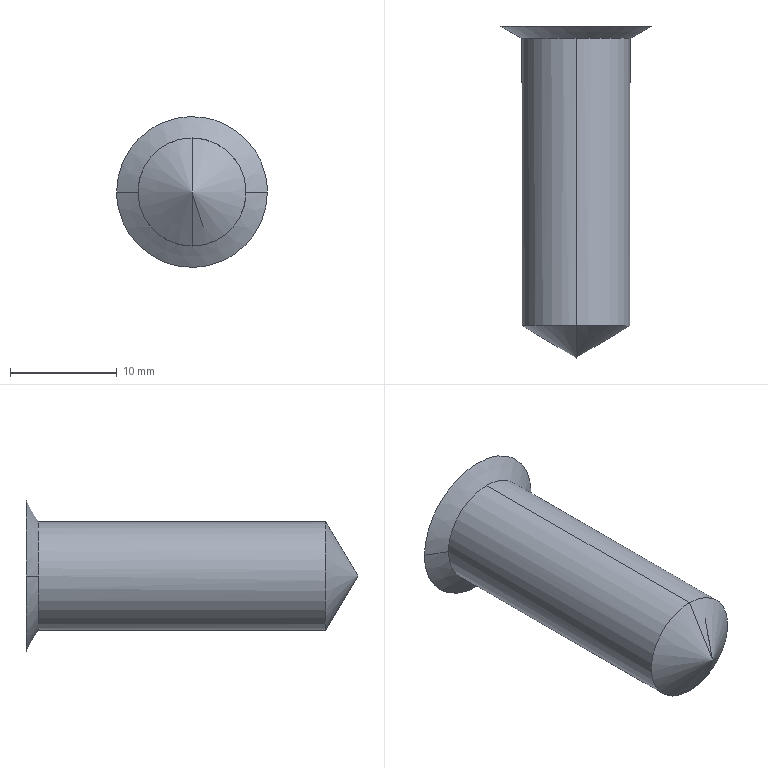Part | NX | features solid 2 | 1 solid | 7 faces | box 14.106 x 31.036 x 14.106 mm | volume 2368 mm3 | cone 4 | cylinder 2 | plane 1 | commonest cylinder face diameters 10.106 x2
STEP:
#1=CARTESIAN_POINT('',(-165.,-29.,-162.053));
#2=VERTEX_POINT('',#1);
#3=CARTESIAN_POINT('',(-165.,-2.155,-162.053));
#4=VERTEX_POINT('',#3);
#5=CARTESIAN_POINT('',(-165.,-29.,-162.053));
#6=CARTESIAN_POINT('',(-165.,-20.052,-162.053));
#7=CARTESIAN_POINT('',(-165.,-11.103,-162.053));
#8=CARTESIAN_POINT('',(-165.,-2.155,-162.053));
#9=B_SPLINE_CURVE_WITH_KNOTS('',3,(#5,#6,#7,#8),.UNSPECIFIED.,.F.,.F.,(4,4),(0.,1.),.UNSPECIFIED.);
#10=EDGE_CURVE('',#2,#4,#9,.T.);
#11=ORIENTED_EDGE('',*,*,#10,.T.);
#12=CARTESIAN_POINT('',(-159.947,-2.155,-157.));
#13=VERTEX_POINT('',#12);
#14=CARTESIAN_POINT('',(-165.,-2.155,-162.053));
#15=CARTESIAN_POINT('',(-163.677,-2.155,-162.053));
#16=CARTESIAN_POINT('',(-161.042,-2.155,-160.958));
#17=CARTESIAN_POINT('',(-159.947,-2.155,-158.323));
#18=CARTESIAN_POINT('',(-159.947,-2.155,-157.));
#19=B_SPLINE_CURVE_WITH_KNOTS('',3,(#14,#15,#16,#17,#18),.UNSPECIFIED.,.F.,.F.,(4,1,4),(0.,0.5,1.),.UNSPECIFIED.);
#20=EDGE_CURVE('',#4,#13,#19,.T.);
#21=ORIENTED_EDGE('',*,*,#20,.T.);
#22=CARTESIAN_POINT('',(-165.,-2.155,-151.947));
#23=VERTEX_POINT('',#22);
#24=CARTESIAN_POINT('',(-159.947,-2.155,-157.));
#25=CARTESIAN_POINT('',(-159.947,-2.155,-155.677));
#26=CARTESIAN_POINT('',(-161.042,-2.155,-153.042));
#27=CARTESIAN_POINT('',(-163.677,-2.155,-151.947));
#28=CARTESIAN_POINT('',(-165.,-2.155,-151.947));
#29=B_SPLINE_CURVE_WITH_KNOTS('',3,(#24,#25,#26,#27,#28),.UNSPECIFIED.,.F.,.F.,(4,1,4),(0.,0.5,1.),.UNSPECIFIED.);
#30=EDGE_CURVE('',#13,#23,#29,.T.);
#31=ORIENTED_EDGE('',*,*,#30,.T.);
#32=CARTESIAN_POINT('',(-165.,-29.,-151.947));
#33=VERTEX_POINT('',#32);
#34=CARTESIAN_POINT('',(-165.,-2.155,-151.947));
#35=CARTESIAN_POINT('',(-165.,-11.103,-151.947));
#36=CARTESIAN_POINT('',(-165.,-20.052,-151.947));
#37=CARTESIAN_POINT('',(-165.,-29.,-151.947));
#38=B_SPLINE_CURVE_WITH_KNOTS('',3,(#34,#35,#36,#37),.UNSPECIFIED.,.F.,.F.,(4,4),(0.,1.),.UNSPECIFIED.);
#39=EDGE_CURVE('',#23,#33,#38,.T.);
#40=ORIENTED_EDGE('',*,*,#39,.T.);
#41=CARTESIAN_POINT('',(-165.,-29.,-151.947));
#42=CARTESIAN_POINT('',(-163.677,-29.,-151.947));
#43=CARTESIAN_POINT('',(-161.042,-29.,-153.04));
#44=CARTESIAN_POINT('',(-159.4,-29.,-157.));
#45=CARTESIAN_POINT('',(-161.042,-29.,-160.96));
#46=CARTESIAN_POINT('',(-163.677,-29.,-162.053));
#47=CARTESIAN_POINT('',(-165.,-29.,-162.053));
#48=B_SPLINE_CURVE_WITH_KNOTS('',3,(#41,#42,#43,#44,#45,#46,#47),.UNSPECIFIED.,.F.,.F.,(4,1,1,1,4),(0.,0.25,0.5,0.75,1.),.UNSPECIFIED.);
#49=EDGE_CURVE('',#33,#2,#48,.T.);
#50=ORIENTED_EDGE('',*,*,#49,.T.);
#51=EDGE_LOOP('',(#11,#21,#31,#40,#50));
#52=FACE_BOUND('',#51,.T.);
#53=CARTESIAN_POINT('',(-165.,-1.,-157.));
#54=DIRECTION('',(0.,-1.,0.));
#55=DIRECTION('',(0.,0.,1.));
#56=AXIS2_PLACEMENT_3D('',#53,#54,#55);
#57=CYLINDRICAL_SURFACE('',#56,5.053);
#58=ADVANCED_FACE('',(#52),#57,.T.);
#59=CARTESIAN_POINT('',(-157.947,-1.,-157.));
#60=VERTEX_POINT('',#59);
#61=CARTESIAN_POINT('',(-157.947,-1.,-157.));
#62=CARTESIAN_POINT('',(-158.614,-1.385,-157.));
#63=CARTESIAN_POINT('',(-159.28,-1.77,-157.));
#64=CARTESIAN_POINT('',(-159.947,-2.155,-157.));
#65=B_SPLINE_CURVE_WITH_KNOTS('',3,(#61,#62,#63,#64),.UNSPECIFIED.,.F.,.F.,(4,4),(0.,1.),.UNSPECIFIED.);
#66=EDGE_CURVE('',#60,#13,#65,.T.);
#67=ORIENTED_EDGE('',*,*,#66,.T.);
#68=ORIENTED_EDGE('',*,*,#20,.F.);
#69=CARTESIAN_POINT('',(-170.053,-2.155,-157.));
#70=VERTEX_POINT('',#69);
#71=CARTESIAN_POINT('',(-170.053,-2.155,-157.));
#72=CARTESIAN_POINT('',(-170.053,-2.155,-158.323));
#73=CARTESIAN_POINT('',(-168.958,-2.155,-160.958));
#74=CARTESIAN_POINT('',(-166.323,-2.155,-162.053));
#75=CARTESIAN_POINT('',(-165.,-2.155,-162.053));
#76=B_SPLINE_CURVE_WITH_KNOTS('',3,(#71,#72,#73,#74,#75),.UNSPECIFIED.,.F.,.F.,(4,1,4),(0.,0.5,1.),.UNSPECIFIED.);
#77=EDGE_CURVE('',#4,#70,#76,.F.);
#78=ORIENTED_EDGE('',*,*,#77,.T.);
#79=CARTESIAN_POINT('',(-172.053,-1.,-157.));
#80=VERTEX_POINT('',#79);
#81=CARTESIAN_POINT('',(-170.053,-2.155,-157.));
#82=CARTESIAN_POINT('',(-170.72,-1.77,-157.));
#83=CARTESIAN_POINT('',(-171.386,-1.385,-157.));
#84=CARTESIAN_POINT('',(-172.053,-1.,-157.));
#85=B_SPLINE_CURVE_WITH_KNOTS('',3,(#81,#82,#83,#84),.UNSPECIFIED.,.F.,.F.,(4,4),(0.,1.),.UNSPECIFIED.);
#86=EDGE_CURVE('',#70,#80,#85,.T.);
#87=ORIENTED_EDGE('',*,*,#86,.T.);
#88=CARTESIAN_POINT('',(-157.947,-1.,-157.));
#89=CARTESIAN_POINT('',(-157.947,-1.,-158.852));
#90=CARTESIAN_POINT('',(-159.473,-1.,-162.522));
#91=CARTESIAN_POINT('',(-165.,-1.,-164.819));
#92=CARTESIAN_POINT('',(-170.527,-1.,-162.521));
#93=CARTESIAN_POINT('',(-172.053,-1.,-158.853));
#94=CARTESIAN_POINT('',(-172.053,-1.,-157.));
#95=B_SPLINE_CURVE_WITH_KNOTS('',3,(#88,#89,#90,#91,#92,#93,#94),.UNSPECIFIED.,.F.,.F.,(4,1,1,1,4),(0.,0.25,0.5,0.75,1.),.UNSPECIFIED.);
#96=EDGE_CURVE('',#80,#60,#95,.F.);
#97=ORIENTED_EDGE('',*,*,#96,.T.);
#98=EDGE_LOOP('',(#67,#68,#78,#87,#97));
#99=FACE_BOUND('',#98,.T.);
#100=CARTESIAN_POINT('',(-165.,-1.,-157.));
#101=DIRECTION('',(0.,1.,0.));
#102=DIRECTION('',(-1.,0.,0.));
#103=AXIS2_PLACEMENT_3D('',#100,#101,#102);
#104=CONICAL_SURFACE('',#103,7.053,1.047);
#105=ADVANCED_FACE('',(#99),#104,.T.);
#106=ORIENTED_EDGE('',*,*,#77,.F.);
#107=ORIENTED_EDGE('',*,*,#10,.F.);
#108=CARTESIAN_POINT('',(-165.,-29.,-162.053));
#109=CARTESIAN_POINT('',(-166.323,-29.,-162.053));
#110=CARTESIAN_POINT('',(-168.958,-29.,-160.96));
#111=CARTESIAN_POINT('',(-170.6,-29.,-157.));
#112=CARTESIAN_POINT('',(-168.958,-29.,-153.04));
#113=CARTESIAN_POINT('',(-166.323,-29.,-151.947));
#114=CARTESIAN_POINT('',(-165.,-29.,-151.947));
#115=B_SPLINE_CURVE_WITH_KNOTS('',3,(#108,#109,#110,#111,#112,#113,#114),.UNSPECIFIED.,.F.,.F.,(4,1,1,1,4),(0.,0.25,0.5,0.75,1.),.UNSPECIFIED.);
#116=EDGE_CURVE('',#2,#33,#115,.T.);
#117=ORIENTED_EDGE('',*,*,#116,.T.);
#118=ORIENTED_EDGE('',*,*,#39,.F.);
#119=CARTESIAN_POINT('',(-165.,-2.155,-151.947));
#120=CARTESIAN_POINT('',(-166.323,-2.155,-151.947));
#121=CARTESIAN_POINT('',(-168.958,-2.155,-153.042));
#122=CARTESIAN_POINT('',(-170.053,-2.155,-155.677));
#123=CARTESIAN_POINT('',(-170.053,-2.155,-157.));
#124=B_SPLINE_CURVE_WITH_KNOTS('',3,(#119,#120,#121,#122,#123),.UNSPECIFIED.,.F.,.F.,(4,1,4),(0.,0.5,1.),.UNSPECIFIED.);
#125=EDGE_CURVE('',#23,#70,#124,.T.);
#126=ORIENTED_EDGE('',*,*,#125,.T.);
#127=EDGE_LOOP('',(#106,#107,#117,#118,#126));
#128=FACE_BOUND('',#127,.T.);
#129=CARTESIAN_POINT('',(-165.,-1.,-157.));
#130=DIRECTION('',(0.,-1.,0.));
#131=DIRECTION('',(0.,0.,1.));
#132=AXIS2_PLACEMENT_3D('',#129,#130,#131);
#133=CYLINDRICAL_SURFACE('',#132,5.053);
#134=ADVANCED_FACE('',(#128),#133,.T.);
#135=CARTESIAN_POINT('',(-165.,-32.036,-157.));
#136=VERTEX_POINT('',#135);
#137=CARTESIAN_POINT('',(-165.,-29.,-151.947));
#138=CARTESIAN_POINT('',(-165.,-30.012,-153.631));
#139=CARTESIAN_POINT('',(-165.,-31.024,-155.316));
#140=CARTESIAN_POINT('',(-165.,-32.036,-157.));
#141=B_SPLINE_CURVE_WITH_KNOTS('',3,(#137,#138,#139,#140),.UNSPECIFIED.,.F.,.F.,(4,4),(0.,1.),.UNSPECIFIED.);
#142=EDGE_CURVE('',#33,#136,#141,.T.);
#143=ORIENTED_EDGE('',*,*,#142,.T.);
#144=CARTESIAN_POINT('',(-165.,-32.036,-157.));
#145=CARTESIAN_POINT('',(-165.,-31.024,-158.684));
#146=CARTESIAN_POINT('',(-165.,-30.012,-160.369));
#147=CARTESIAN_POINT('',(-165.,-29.,-162.053));
#148=B_SPLINE_CURVE_WITH_KNOTS('',3,(#144,#145,#146,#147),.UNSPECIFIED.,.F.,.F.,(4,4),(0.,1.),.UNSPECIFIED.);
#149=EDGE_CURVE('',#136,#2,#148,.T.);
#150=ORIENTED_EDGE('',*,*,#149,.T.);
#151=ORIENTED_EDGE('',*,*,#49,.F.);
#152=EDGE_LOOP('',(#143,#150,#151));
#153=FACE_BOUND('',#152,.T.);
#154=CARTESIAN_POINT('',(-165.,-29.,-157.));
#155=DIRECTION('',(0.,1.,0.));
#156=DIRECTION('',(0.,0.,-1.));
#157=AXIS2_PLACEMENT_3D('',#154,#155,#156);
#158=CONICAL_SURFACE('',#157,5.053,1.03);
#159=ADVANCED_FACE('',(#153),#158,.T.);
#160=ORIENTED_EDGE('',*,*,#30,.F.);
#161=ORIENTED_EDGE('',*,*,#66,.F.);
#162=CARTESIAN_POINT('',(-172.053,-1.,-157.));
#163=CARTESIAN_POINT('',(-172.053,-1.,-155.148));
#164=CARTESIAN_POINT('',(-170.527,-1.,-151.478));
#165=CARTESIAN_POINT('',(-165.,-1.,-149.181));
#166=CARTESIAN_POINT('',(-159.473,-1.,-151.479));
#167=CARTESIAN_POINT('',(-157.947,-1.,-155.147));
#168=CARTESIAN_POINT('',(-157.947,-1.,-157.));
#169=B_SPLINE_CURVE_WITH_KNOTS('',3,(#162,#163,#164,#165,#166,#167,#168),.UNSPECIFIED.,.F.,.F.,(4,1,1,1,4),(0.,0.25,0.5,0.75,1.),.UNSPECIFIED.);
#170=EDGE_CURVE('',#60,#80,#169,.F.);
#171=ORIENTED_EDGE('',*,*,#170,.T.);
#172=ORIENTED_EDGE('',*,*,#86,.F.);
#173=ORIENTED_EDGE('',*,*,#125,.F.);
#174=EDGE_LOOP('',(#160,#161,#171,#172,#173));
#175=FACE_BOUND('',#174,.T.);
#176=CARTESIAN_POINT('',(-165.,-1.,-157.));
#177=DIRECTION('',(0.,1.,0.));
#178=DIRECTION('',(-1.,0.,0.));
#179=AXIS2_PLACEMENT_3D('',#176,#177,#178);
#180=CONICAL_SURFACE('',#179,7.053,1.047);
#181=ADVANCED_FACE('',(#175),#180,.T.);
#182=ORIENTED_EDGE('',*,*,#170,.F.);
#183=ORIENTED_EDGE('',*,*,#96,.F.);
#184=EDGE_LOOP('',(#182,#183));
#185=FACE_BOUND('',#184,.T.);
#186=CARTESIAN_POINT('',(-165.,-1.,-157.));
#187=DIRECTION('',(0.,1.,0.));
#188=DIRECTION('',(0.,0.,-1.));
#189=AXIS2_PLACEMENT_3D('',#186,#187,#188);
#190=PLANE('',#189);
#191=ADVANCED_FACE('',(#185),#190,.T.);
#192=ORIENTED_EDGE('',*,*,#149,.F.);
#193=ORIENTED_EDGE('',*,*,#142,.F.);
#194=ORIENTED_EDGE('',*,*,#116,.F.);
#195=EDGE_LOOP('',(#192,#193,#194));
#196=FACE_BOUND('',#195,.T.);
#197=CARTESIAN_POINT('',(-165.,-29.,-157.));
#198=DIRECTION('',(0.,1.,0.));
#199=DIRECTION('',(0.,0.,-1.));
#200=AXIS2_PLACEMENT_3D('',#197,#198,#199);
#201=CONICAL_SURFACE('',#200,5.053,1.03);
#202=ADVANCED_FACE('',(#196),#201,.T.);
#203=CLOSED_SHELL('',(#58,#105,#134,#159,#181,#191,#202));
#204=MANIFOLD_SOLID_BREP('',#203);
#205=(LENGTH_UNIT()NAMED_UNIT(*)SI_UNIT(.MILLI.,.METRE.));
#206=UNCERTAINTY_MEASURE_WITH_UNIT(LENGTH_MEASURE(0.0508),#205,'','');
#207=(NAMED_UNIT(*)PLANE_ANGLE_UNIT()SI_UNIT($,.RADIAN.));
#208=(NAMED_UNIT(*)SI_UNIT($,.STERADIAN.)SOLID_ANGLE_UNIT());
#209=(GEOMETRIC_REPRESENTATION_CONTEXT(3)GLOBAL_UNCERTAINTY_ASSIGNED_CONTEXT((#206))GLOBAL_UNIT_ASSIGNED_CONTEXT((#205,#207,#208))REPRESENTATION_CONTEXT('',''));
#210=ADVANCED_BREP_SHAPE_REPRESENTATION('',(#204),#209);